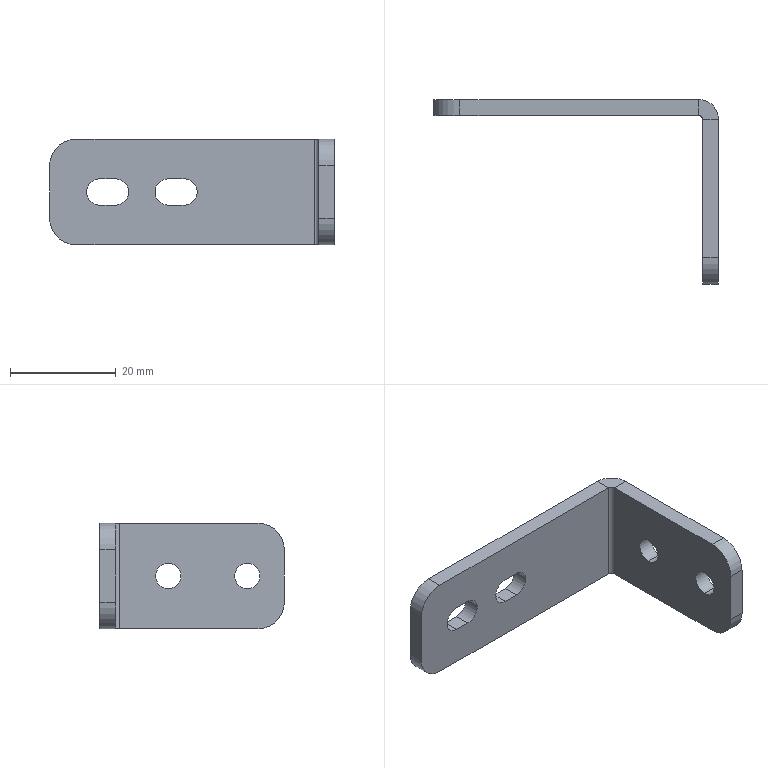Part | SolidWorks | features Fillet 1, FlatPattern 1, HoleWzd 1, ICE 1, SMBaseFlange 1, SheetMetal 1 | 1 solid | 30 faces | box 54 x 35 x 20 mm | volume 4722 mm3 | plane 16 | cylinder 14 | commonest cylinder face diameters 4.8 x4 5 x4 10 x4 1.473 x1 7.473 x1
STEP:
#1=CARTESIAN_POINT('',(54.,-13.,12.4));
#2=VERTEX_POINT('',#1);
#3=CARTESIAN_POINT('',(54.,-13.,7.6));
#4=VERTEX_POINT('',#3);
#5=CARTESIAN_POINT('',(54.,-13.,10.));
#6=DIRECTION('',(1.,0.,0.));
#7=DIRECTION('',(0.,1.,0.));
#8=AXIS2_PLACEMENT_3D('',#5,#6,#7);
#9=CIRCLE('',#8,2.4);
#10=EDGE_CURVE('',#2,#4,#9,.T.);
#11=ORIENTED_EDGE('',*,*,#10,.T.);
#12=CARTESIAN_POINT('',(51.,-13.,7.6));
#13=VERTEX_POINT('',#12);
#14=CARTESIAN_POINT('',(51.,-13.,7.6));
#15=DIRECTION('',(-1.,0.,0.));
#16=VECTOR('',#15,1000.);
#17=LINE('',#14,#16);
#18=EDGE_CURVE('',#4,#13,#17,.T.);
#19=ORIENTED_EDGE('',*,*,#18,.T.);
#20=CARTESIAN_POINT('',(51.,-13.,12.4));
#21=VERTEX_POINT('',#20);
#22=CARTESIAN_POINT('',(51.,-13.,10.));
#23=DIRECTION('',(-1.,0.,0.));
#24=DIRECTION('',(0.,0.,1.));
#25=AXIS2_PLACEMENT_3D('',#22,#23,#24);
#26=CIRCLE('',#25,2.4);
#27=EDGE_CURVE('',#13,#21,#26,.T.);
#28=ORIENTED_EDGE('',*,*,#27,.T.);
#29=CARTESIAN_POINT('',(51.,-13.,12.4));
#30=DIRECTION('',(-1.,0.,0.));
#31=VECTOR('',#30,1000.);
#32=LINE('',#29,#31);
#33=EDGE_CURVE('',#2,#21,#32,.T.);
#34=ORIENTED_EDGE('',*,*,#33,.F.);
#35=EDGE_LOOP('',(#11,#19,#28,#34));
#36=FACE_OUTER_BOUND('',#35,.T.);
#37=CARTESIAN_POINT('',(51.,-13.,10.));
#38=DIRECTION('',(-1.,0.,0.));
#39=DIRECTION('',(0.,0.,1.));
#40=AXIS2_PLACEMENT_3D('',#37,#38,#39);
#41=CYLINDRICAL_SURFACE('',#40,2.4);
#42=ADVANCED_FACE('',(#36),#41,.F.);
#43=CARTESIAN_POINT('',(54.,-28.,12.4));
#44=VERTEX_POINT('',#43);
#45=CARTESIAN_POINT('',(54.,-28.,7.6));
#46=VERTEX_POINT('',#45);
#47=CARTESIAN_POINT('',(54.,-28.,10.));
#48=DIRECTION('',(1.,0.,0.));
#49=DIRECTION('',(0.,1.,0.));
#50=AXIS2_PLACEMENT_3D('',#47,#48,#49);
#51=CIRCLE('',#50,2.4);
#52=EDGE_CURVE('',#44,#46,#51,.T.);
#53=ORIENTED_EDGE('',*,*,#52,.T.);
#54=CARTESIAN_POINT('',(51.,-28.,7.6));
#55=VERTEX_POINT('',#54);
#56=CARTESIAN_POINT('',(51.,-28.,7.6));
#57=DIRECTION('',(-1.,0.,0.));
#58=VECTOR('',#57,1000.);
#59=LINE('',#56,#58);
#60=EDGE_CURVE('',#46,#55,#59,.T.);
#61=ORIENTED_EDGE('',*,*,#60,.T.);
#62=CARTESIAN_POINT('',(51.,-28.,12.4));
#63=VERTEX_POINT('',#62);
#64=CARTESIAN_POINT('',(51.,-28.,10.));
#65=DIRECTION('',(-1.,0.,0.));
#66=DIRECTION('',(0.,0.,1.));
#67=AXIS2_PLACEMENT_3D('',#64,#65,#66);
#68=CIRCLE('',#67,2.4);
#69=EDGE_CURVE('',#55,#63,#68,.T.);
#70=ORIENTED_EDGE('',*,*,#69,.T.);
#71=CARTESIAN_POINT('',(51.,-28.,12.4));
#72=DIRECTION('',(-1.,0.,0.));
#73=VECTOR('',#72,1000.);
#74=LINE('',#71,#73);
#75=EDGE_CURVE('',#44,#63,#74,.T.);
#76=ORIENTED_EDGE('',*,*,#75,.F.);
#77=EDGE_LOOP('',(#53,#61,#70,#76));
#78=FACE_OUTER_BOUND('',#77,.T.);
#79=CARTESIAN_POINT('',(51.,-28.,10.));
#80=DIRECTION('',(-1.,0.,0.));
#81=DIRECTION('',(0.,0.,1.));
#82=AXIS2_PLACEMENT_3D('',#79,#80,#81);
#83=CYLINDRICAL_SURFACE('',#82,2.4);
#84=ADVANCED_FACE('',(#78),#83,.F.);
#85=CARTESIAN_POINT('',(54.,-3.737,20.));
#86=VERTEX_POINT('',#85);
#87=CARTESIAN_POINT('',(51.,-3.737,20.));
#88=VERTEX_POINT('',#87);
#89=CARTESIAN_POINT('',(54.,-3.737,20.));
#90=DIRECTION('',(-1.,0.,0.));
#91=VECTOR('',#90,1000.);
#92=LINE('',#89,#91);
#93=EDGE_CURVE('',#86,#88,#92,.T.);
#94=ORIENTED_EDGE('',*,*,#93,.F.);
#95=CARTESIAN_POINT('',(50.263,0.,20.));
#96=VERTEX_POINT('',#95);
#97=CARTESIAN_POINT('',(50.263,-3.737,20.));
#98=DIRECTION('',(0.,0.,-1.));
#99=DIRECTION('',(1.,0.,0.));
#100=AXIS2_PLACEMENT_3D('',#97,#98,#99);
#101=CIRCLE('',#100,3.737);
#102=EDGE_CURVE('',#96,#86,#101,.T.);
#103=ORIENTED_EDGE('',*,*,#102,.F.);
#104=CARTESIAN_POINT('',(50.263,-3.,20.));
#105=VERTEX_POINT('',#104);
#106=CARTESIAN_POINT('',(50.263,-3.,20.));
#107=DIRECTION('',(0.,1.,0.));
#108=VECTOR('',#107,1000.);
#109=LINE('',#106,#108);
#110=EDGE_CURVE('',#105,#96,#109,.T.);
#111=ORIENTED_EDGE('',*,*,#110,.F.);
#112=CARTESIAN_POINT('',(50.263,-3.737,20.));
#113=DIRECTION('',(0.,0.,-1.));
#114=DIRECTION('',(1.,0.,0.));
#115=AXIS2_PLACEMENT_3D('',#112,#113,#114);
#116=CIRCLE('',#115,0.7366);
#117=EDGE_CURVE('',#105,#88,#116,.T.);
#118=ORIENTED_EDGE('',*,*,#117,.T.);
#119=EDGE_LOOP('',(#94,#103,#111,#118));
#120=FACE_OUTER_BOUND('',#119,.T.);
#121=CARTESIAN_POINT('',(54.,-3.737,20.));
#122=DIRECTION('',(0.,0.,1.));
#123=DIRECTION('',(1.,0.,0.));
#124=AXIS2_PLACEMENT_3D('',#121,#122,#123);
#125=PLANE('',#124);
#126=ADVANCED_FACE('',(#120),#125,.T.);
#127=CARTESIAN_POINT('',(51.,-30.,20.));
#128=VERTEX_POINT('',#127);
#129=CARTESIAN_POINT('',(51.,0.,20.));
#130=DIRECTION('',(0.,-1.,0.));
#131=VECTOR('',#130,1000.);
#132=LINE('',#129,#131);
#133=EDGE_CURVE('',#88,#128,#132,.T.);
#134=ORIENTED_EDGE('',*,*,#133,.T.);
#135=CARTESIAN_POINT('',(54.,-30.,20.));
#136=VERTEX_POINT('',#135);
#137=CARTESIAN_POINT('',(50.263,-30.,20.));
#138=DIRECTION('',(1.,0.,0.));
#139=VECTOR('',#138,1000.);
#140=LINE('',#137,#139);
#141=EDGE_CURVE('',#128,#136,#140,.T.);
#142=ORIENTED_EDGE('',*,*,#141,.T.);
#143=CARTESIAN_POINT('',(54.,0.,20.));
#144=DIRECTION('',(0.,-1.,0.));
#145=VECTOR('',#144,1000.);
#146=LINE('',#143,#145);
#147=EDGE_CURVE('',#86,#136,#146,.T.);
#148=ORIENTED_EDGE('',*,*,#147,.F.);
#149=ORIENTED_EDGE('',*,*,#93,.T.);
#150=EDGE_LOOP('',(#134,#142,#148,#149));
#151=FACE_OUTER_BOUND('',#150,.T.);
#152=CARTESIAN_POINT('',(50.263,-3.,20.));
#153=DIRECTION('',(0.,0.,1.));
#154=DIRECTION('',(1.,0.,0.));
#155=AXIS2_PLACEMENT_3D('',#152,#153,#154);
#156=PLANE('',#155);
#157=ADVANCED_FACE('',(#151),#156,.T.);
#158=CARTESIAN_POINT('',(50.263,0.,0.));
#159=VERTEX_POINT('',#158);
#160=CARTESIAN_POINT('',(50.263,-3.,0.));
#161=VERTEX_POINT('',#160);
#162=CARTESIAN_POINT('',(50.263,0.,0.));
#163=DIRECTION('',(0.,-1.,0.));
#164=VECTOR('',#163,1000.);
#165=LINE('',#162,#164);
#166=EDGE_CURVE('',#159,#161,#165,.T.);
#167=ORIENTED_EDGE('',*,*,#166,.F.);
#168=CARTESIAN_POINT('',(54.,-3.737,0.));
#169=VERTEX_POINT('',#168);
#170=CARTESIAN_POINT('',(50.263,-3.737,0.));
#171=DIRECTION('',(0.,0.,-1.));
#172=DIRECTION('',(1.,0.,0.));
#173=AXIS2_PLACEMENT_3D('',#170,#171,#172);
#174=CIRCLE('',#173,3.737);
#175=EDGE_CURVE('',#159,#169,#174,.T.);
#176=ORIENTED_EDGE('',*,*,#175,.T.);
#177=CARTESIAN_POINT('',(51.,-3.737,0.));
#178=VERTEX_POINT('',#177);
#179=CARTESIAN_POINT('',(51.,-3.737,0.));
#180=DIRECTION('',(1.,0.,0.));
#181=VECTOR('',#180,1000.);
#182=LINE('',#179,#181);
#183=EDGE_CURVE('',#178,#169,#182,.T.);
#184=ORIENTED_EDGE('',*,*,#183,.F.);
#185=CARTESIAN_POINT('',(50.263,-3.737,0.));
#186=DIRECTION('',(0.,0.,-1.));
#187=DIRECTION('',(1.,0.,0.));
#188=AXIS2_PLACEMENT_3D('',#185,#186,#187);
#189=CIRCLE('',#188,0.7366);
#190=EDGE_CURVE('',#161,#178,#189,.T.);
#191=ORIENTED_EDGE('',*,*,#190,.F.);
#192=EDGE_LOOP('',(#167,#176,#184,#191));
#193=FACE_OUTER_BOUND('',#192,.T.);
#194=CARTESIAN_POINT('',(50.263,0.,0.));
#195=DIRECTION('',(0.,0.,-1.));
#196=DIRECTION('',(-1.,0.,0.));
#197=AXIS2_PLACEMENT_3D('',#194,#195,#196);
#198=PLANE('',#197);
#199=ADVANCED_FACE('',(#193),#198,.T.);
#200=CARTESIAN_POINT('',(5.,-3.,0.));
#201=VERTEX_POINT('',#200);
#202=CARTESIAN_POINT('',(0.,-3.,0.));
#203=DIRECTION('',(1.,0.,0.));
#204=VECTOR('',#203,1000.);
#205=LINE('',#202,#204);
#206=EDGE_CURVE('',#201,#161,#205,.T.);
#207=ORIENTED_EDGE('',*,*,#206,.F.);
#208=CARTESIAN_POINT('',(5.,0.,0.));
#209=VERTEX_POINT('',#208);
#210=CARTESIAN_POINT('',(5.,-3.737,0.));
#211=DIRECTION('',(0.,1.,0.));
#212=VECTOR('',#211,1000.);
#213=LINE('',#210,#212);
#214=EDGE_CURVE('',#201,#209,#213,.T.);
#215=ORIENTED_EDGE('',*,*,#214,.T.);
#216=CARTESIAN_POINT('',(0.,0.,0.));
#217=DIRECTION('',(1.,0.,0.));
#218=VECTOR('',#217,1000.);
#219=LINE('',#216,#218);
#220=EDGE_CURVE('',#209,#159,#219,.T.);
#221=ORIENTED_EDGE('',*,*,#220,.T.);
#222=ORIENTED_EDGE('',*,*,#166,.T.);
#223=EDGE_LOOP('',(#207,#215,#221,#222));
#224=FACE_OUTER_BOUND('',#223,.T.);
#225=CARTESIAN_POINT('',(51.,-3.737,0.));
#226=DIRECTION('',(0.,0.,-1.));
#227=DIRECTION('',(-1.,0.,0.));
#228=AXIS2_PLACEMENT_3D('',#225,#226,#227);
#229=PLANE('',#228);
#230=ADVANCED_FACE('',(#224),#229,.T.);
#231=CARTESIAN_POINT('',(51.,-13.,10.));
#232=DIRECTION('',(-1.,0.,0.));
#233=DIRECTION('',(0.,0.,1.));
#234=AXIS2_PLACEMENT_3D('',#231,#232,#233);
#235=CIRCLE('',#234,2.4);
#236=EDGE_CURVE('',#21,#13,#235,.T.);
#237=ORIENTED_EDGE('',*,*,#236,.F.);
#238=ORIENTED_EDGE('',*,*,#27,.F.);
#239=EDGE_LOOP('',(#237,#238));
#240=FACE_BOUND('',#239,.T.);
#241=CARTESIAN_POINT('',(51.,-28.,10.));
#242=DIRECTION('',(-1.,0.,0.));
#243=DIRECTION('',(0.,0.,1.));
#244=AXIS2_PLACEMENT_3D('',#241,#242,#243);
#245=CIRCLE('',#244,2.4);
#246=EDGE_CURVE('',#63,#55,#245,.T.);
#247=ORIENTED_EDGE('',*,*,#246,.F.);
#248=ORIENTED_EDGE('',*,*,#69,.F.);
#249=EDGE_LOOP('',(#247,#248));
#250=FACE_BOUND('',#249,.T.);
#251=CARTESIAN_POINT('',(51.,-35.,15.));
#252=VERTEX_POINT('',#251);
#253=CARTESIAN_POINT('',(51.,-35.,5.));
#254=VERTEX_POINT('',#253);
#255=CARTESIAN_POINT('',(51.,-35.,20.));
#256=DIRECTION('',(0.,0.,-1.));
#257=VECTOR('',#256,1000.);
#258=LINE('',#255,#257);
#259=EDGE_CURVE('',#252,#254,#258,.T.);
#260=ORIENTED_EDGE('',*,*,#259,.F.);
#261=CARTESIAN_POINT('',(51.,-30.,15.));
#262=DIRECTION('',(-1.,0.,0.));
#263=DIRECTION('',(0.,1.,0.));
#264=AXIS2_PLACEMENT_3D('',#261,#262,#263);
#265=CIRCLE('',#264,5.);
#266=EDGE_CURVE('',#252,#128,#265,.T.);
#267=ORIENTED_EDGE('',*,*,#266,.T.);
#268=ORIENTED_EDGE('',*,*,#133,.F.);
#269=CARTESIAN_POINT('',(51.,-3.737,20.));
#270=DIRECTION('',(0.,0.,-1.));
#271=VECTOR('',#270,1000.);
#272=LINE('',#269,#271);
#273=EDGE_CURVE('',#88,#178,#272,.T.);
#274=ORIENTED_EDGE('',*,*,#273,.T.);
#275=CARTESIAN_POINT('',(51.,-30.,0.));
#276=VERTEX_POINT('',#275);
#277=CARTESIAN_POINT('',(51.,0.,0.));
#278=DIRECTION('',(0.,-1.,0.));
#279=VECTOR('',#278,1000.);
#280=LINE('',#277,#279);
#281=EDGE_CURVE('',#178,#276,#280,.T.);
#282=ORIENTED_EDGE('',*,*,#281,.T.);
#283=CARTESIAN_POINT('',(51.,-30.,5.));
#284=DIRECTION('',(-1.,0.,0.));
#285=DIRECTION('',(0.,1.,0.));
#286=AXIS2_PLACEMENT_3D('',#283,#284,#285);
#287=CIRCLE('',#286,5.);
#288=EDGE_CURVE('',#276,#254,#287,.T.);
#289=ORIENTED_EDGE('',*,*,#288,.T.);
#290=EDGE_LOOP('',(#260,#267,#268,#274,#282,#289));
#291=FACE_OUTER_BOUND('',#290,.T.);
#292=CARTESIAN_POINT('',(51.,0.,20.));
#293=DIRECTION('',(1.,0.,0.));
#294=DIRECTION('',(0.,1.,0.));
#295=AXIS2_PLACEMENT_3D('',#292,#293,#294);
#296=PLANE('',#295);
#297=ADVANCED_FACE('',(#240,#250,#291),#296,.F.);
#298=CARTESIAN_POINT('',(54.,-35.,15.));
#299=VERTEX_POINT('',#298);
#300=CARTESIAN_POINT('',(54.,-35.,5.));
#301=VERTEX_POINT('',#300);
#302=CARTESIAN_POINT('',(54.,-35.,20.));
#303=DIRECTION('',(0.,0.,-1.));
#304=VECTOR('',#303,1000.);
#305=LINE('',#302,#304);
#306=EDGE_CURVE('',#299,#301,#305,.T.);
#307=ORIENTED_EDGE('',*,*,#306,.F.);
#308=CARTESIAN_POINT('',(54.,-35.,15.));
#309=DIRECTION('',(-1.,0.,0.));
#310=VECTOR('',#309,1000.);
#311=LINE('',#308,#310);
#312=EDGE_CURVE('',#299,#252,#311,.T.);
#313=ORIENTED_EDGE('',*,*,#312,.T.);
#314=ORIENTED_EDGE('',*,*,#259,.T.);
#315=CARTESIAN_POINT('',(54.,-35.,5.));
#316=DIRECTION('',(1.,0.,0.));
#317=VECTOR('',#316,1000.);
#318=LINE('',#315,#317);
#319=EDGE_CURVE('',#254,#301,#318,.T.);
#320=ORIENTED_EDGE('',*,*,#319,.T.);
#321=EDGE_LOOP('',(#307,#313,#314,#320));
#322=FACE_OUTER_BOUND('',#321,.T.);
#323=CARTESIAN_POINT('',(54.,-35.,20.));
#324=DIRECTION('',(0.,-1.,0.));
#325=DIRECTION('',(0.,0.,-1.));
#326=AXIS2_PLACEMENT_3D('',#323,#324,#325);
#327=PLANE('',#326);
#328=ADVANCED_FACE('',(#322),#327,.T.);
#329=ORIENTED_EDGE('',*,*,#10,.F.);
#330=CARTESIAN_POINT('',(54.,-13.,10.));
#331=DIRECTION('',(1.,0.,0.));
#332=DIRECTION('',(0.,1.,0.));
#333=AXIS2_PLACEMENT_3D('',#330,#331,#332);
#334=CIRCLE('',#333,2.4);
#335=EDGE_CURVE('',#4,#2,#334,.T.);
#336=ORIENTED_EDGE('',*,*,#335,.F.);
#337=EDGE_LOOP('',(#329,#336));
#338=FACE_BOUND('',#337,.T.);
#339=ORIENTED_EDGE('',*,*,#52,.F.);
#340=CARTESIAN_POINT('',(54.,-28.,10.));
#341=DIRECTION('',(1.,0.,0.));
#342=DIRECTION('',(0.,1.,0.));
#343=AXIS2_PLACEMENT_3D('',#340,#341,#342);
#344=CIRCLE('',#343,2.4);
#345=EDGE_CURVE('',#46,#44,#344,.T.);
#346=ORIENTED_EDGE('',*,*,#345,.F.);
#347=EDGE_LOOP('',(#339,#346));
#348=FACE_BOUND('',#347,.T.);
#349=ORIENTED_EDGE('',*,*,#147,.T.);
#350=CARTESIAN_POINT('',(54.,-30.,15.));
#351=DIRECTION('',(1.,0.,0.));
#352=DIRECTION('',(0.,1.,0.));
#353=AXIS2_PLACEMENT_3D('',#350,#351,#352);
#354=CIRCLE('',#353,5.);
#355=EDGE_CURVE('',#136,#299,#354,.T.);
#356=ORIENTED_EDGE('',*,*,#355,.T.);
#357=ORIENTED_EDGE('',*,*,#306,.T.);
#358=CARTESIAN_POINT('',(54.,-30.,0.));
#359=VERTEX_POINT('',#358);
#360=CARTESIAN_POINT('',(54.,-30.,5.));
#361=DIRECTION('',(1.,0.,0.));
#362=DIRECTION('',(0.,1.,0.));
#363=AXIS2_PLACEMENT_3D('',#360,#361,#362);
#364=CIRCLE('',#363,5.);
#365=EDGE_CURVE('',#301,#359,#364,.T.);
#366=ORIENTED_EDGE('',*,*,#365,.T.);
#367=CARTESIAN_POINT('',(54.,0.,0.));
#368=DIRECTION('',(0.,-1.,0.));
#369=VECTOR('',#368,1000.);
#370=LINE('',#367,#369);
#371=EDGE_CURVE('',#169,#359,#370,.T.);
#372=ORIENTED_EDGE('',*,*,#371,.F.);
#373=CARTESIAN_POINT('',(54.,-3.737,20.));
#374=DIRECTION('',(0.,0.,-1.));
#375=VECTOR('',#374,1000.);
#376=LINE('',#373,#375);
#377=EDGE_CURVE('',#86,#169,#376,.T.);
#378=ORIENTED_EDGE('',*,*,#377,.F.);
#379=EDGE_LOOP('',(#349,#356,#357,#366,#372,#378));
#380=FACE_OUTER_BOUND('',#379,.T.);
#381=CARTESIAN_POINT('',(54.,0.,20.));
#382=DIRECTION('',(1.,0.,0.));
#383=DIRECTION('',(0.,1.,0.));
#384=AXIS2_PLACEMENT_3D('',#381,#382,#383);
#385=PLANE('',#384);
#386=ADVANCED_FACE('',(#338,#348,#380),#385,.T.);
#387=ORIENTED_EDGE('',*,*,#175,.F.);
#388=CARTESIAN_POINT('',(50.263,0.,20.));
#389=DIRECTION('',(0.,0.,-1.));
#390=VECTOR('',#389,1000.);
#391=LINE('',#388,#390);
#392=EDGE_CURVE('',#96,#159,#391,.T.);
#393=ORIENTED_EDGE('',*,*,#392,.F.);
#394=ORIENTED_EDGE('',*,*,#102,.T.);
#395=ORIENTED_EDGE('',*,*,#377,.T.);
#396=EDGE_LOOP('',(#387,#393,#394,#395));
#397=FACE_OUTER_BOUND('',#396,.T.);
#398=CARTESIAN_POINT('',(50.263,-3.737,20.));
#399=DIRECTION('',(0.,0.,-1.));
#400=DIRECTION('',(-1.,0.,0.));
#401=AXIS2_PLACEMENT_3D('',#398,#399,#400);
#402=CYLINDRICAL_SURFACE('',#401,3.737);
#403=ADVANCED_FACE('',(#397),#402,.T.);
#404=CARTESIAN_POINT('',(9.5,0.,7.5));
#405=VERTEX_POINT('',#404);
#406=CARTESIAN_POINT('',(9.5,0.,12.5));
#407=VERTEX_POINT('',#406);
#408=CARTESIAN_POINT('',(9.5,0.,10.));
#409=DIRECTION('',(0.,1.,0.));
#410=DIRECTION('',(0.,0.,1.));
#411=AXIS2_PLACEMENT_3D('',#408,#409,#410);
#412=CIRCLE('',#411,2.5);
#413=EDGE_CURVE('',#405,#407,#412,.T.);
#414=ORIENTED_EDGE('',*,*,#413,.F.);
#415=CARTESIAN_POINT('',(12.5,0.,7.5));
#416=VERTEX_POINT('',#415);
#417=CARTESIAN_POINT('',(9.5,0.,7.5));
#418=DIRECTION('',(-1.,0.,0.));
#419=VECTOR('',#418,1000.);
#420=LINE('',#417,#419);
#421=EDGE_CURVE('',#416,#405,#420,.T.);
#422=ORIENTED_EDGE('',*,*,#421,.F.);
#423=CARTESIAN_POINT('',(12.5,0.,12.5));
#424=VERTEX_POINT('',#423);
#425=CARTESIAN_POINT('',(12.5,0.,10.));
#426=DIRECTION('',(0.,1.,0.));
#427=DIRECTION('',(0.,0.,1.));
#428=AXIS2_PLACEMENT_3D('',#425,#426,#427);
#429=CIRCLE('',#428,2.5);
#430=EDGE_CURVE('',#424,#416,#429,.T.);
#431=ORIENTED_EDGE('',*,*,#430,.F.);
#432=CARTESIAN_POINT('',(9.5,0.,12.5));
#433=DIRECTION('',(1.,0.,0.));
#434=VECTOR('',#433,1000.);
#435=LINE('',#432,#434);
#436=EDGE_CURVE('',#407,#424,#435,.T.);
#437=ORIENTED_EDGE('',*,*,#436,.F.);
#438=EDGE_LOOP('',(#414,#422,#431,#437));
#439=FACE_BOUND('',#438,.T.);
#440=CARTESIAN_POINT('',(25.5,0.,12.5));
#441=VERTEX_POINT('',#440);
#442=CARTESIAN_POINT('',(25.5,0.,7.5));
#443=VERTEX_POINT('',#442);
#444=CARTESIAN_POINT('',(25.5,0.,10.));
#445=DIRECTION('',(0.,1.,0.));
#446=DIRECTION('',(0.,0.,-1.));
#447=AXIS2_PLACEMENT_3D('',#444,#445,#446);
#448=CIRCLE('',#447,2.5);
#449=EDGE_CURVE('',#441,#443,#448,.T.);
#450=ORIENTED_EDGE('',*,*,#449,.F.);
#451=CARTESIAN_POINT('',(22.5,0.,12.5));
#452=VERTEX_POINT('',#451);
#453=CARTESIAN_POINT('',(25.5,0.,12.5));
#454=DIRECTION('',(1.,0.,0.));
#455=VECTOR('',#454,1000.);
#456=LINE('',#453,#455);
#457=EDGE_CURVE('',#452,#441,#456,.T.);
#458=ORIENTED_EDGE('',*,*,#457,.F.);
#459=CARTESIAN_POINT('',(22.5,0.,7.5));
#460=VERTEX_POINT('',#459);
#461=CARTESIAN_POINT('',(22.5,0.,10.));
#462=DIRECTION('',(0.,1.,0.));
#463=DIRECTION('',(0.,0.,-1.));
#464=AXIS2_PLACEMENT_3D('',#461,#462,#463);
#465=CIRCLE('',#464,2.5);
#466=EDGE_CURVE('',#460,#452,#465,.T.);
#467=ORIENTED_EDGE('',*,*,#466,.F.);
#468=CARTESIAN_POINT('',(25.5,0.,7.5));
#469=DIRECTION('',(-1.,0.,0.));
#470=VECTOR('',#469,1000.);
#471=LINE('',#468,#470);
#472=EDGE_CURVE('',#443,#460,#471,.T.);
#473=ORIENTED_EDGE('',*,*,#472,.F.);
#474=EDGE_LOOP('',(#450,#458,#467,#473));
#475=FACE_BOUND('',#474,.T.);
#476=CARTESIAN_POINT('',(0.,0.,15.));
#477=VERTEX_POINT('',#476);
#478=CARTESIAN_POINT('',(0.,0.,5.));
#479=VERTEX_POINT('',#478);
#480=CARTESIAN_POINT('',(0.,0.,20.));
#481=DIRECTION('',(0.,0.,-1.));
#482=VECTOR('',#481,1000.);
#483=LINE('',#480,#482);
#484=EDGE_CURVE('',#477,#479,#483,.T.);
#485=ORIENTED_EDGE('',*,*,#484,.F.);
#486=CARTESIAN_POINT('',(5.,0.,20.));
#487=VERTEX_POINT('',#486);
#488=CARTESIAN_POINT('',(5.,0.,15.));
#489=DIRECTION('',(0.,1.,0.));
#490=DIRECTION('',(0.,0.,1.));
#491=AXIS2_PLACEMENT_3D('',#488,#489,#490);
#492=CIRCLE('',#491,5.);
#493=EDGE_CURVE('',#477,#487,#492,.T.);
#494=ORIENTED_EDGE('',*,*,#493,.T.);
#495=CARTESIAN_POINT('',(0.,0.,20.));
#496=DIRECTION('',(1.,0.,0.));
#497=VECTOR('',#496,1000.);
#498=LINE('',#495,#497);
#499=EDGE_CURVE('',#487,#96,#498,.T.);
#500=ORIENTED_EDGE('',*,*,#499,.T.);
#501=ORIENTED_EDGE('',*,*,#392,.T.);
#502=ORIENTED_EDGE('',*,*,#220,.F.);
#503=CARTESIAN_POINT('',(5.,0.,5.));
#504=DIRECTION('',(0.,1.,0.));
#505=DIRECTION('',(0.,0.,1.));
#506=AXIS2_PLACEMENT_3D('',#503,#504,#505);
#507=CIRCLE('',#506,5.);
#508=EDGE_CURVE('',#209,#479,#507,.T.);
#509=ORIENTED_EDGE('',*,*,#508,.T.);
#510=EDGE_LOOP('',(#485,#494,#500,#501,#502,#509));
#511=FACE_OUTER_BOUND('',#510,.T.);
#512=CARTESIAN_POINT('',(0.,0.,20.));
#513=DIRECTION('',(0.,1.,0.));
#514=DIRECTION('',(0.,0.,1.));
#515=AXIS2_PLACEMENT_3D('',#512,#513,#514);
#516=PLANE('',#515);
#517=ADVANCED_FACE('',(#439,#475,#511),#516,.T.);
#518=CARTESIAN_POINT('',(0.,-3.,15.));
#519=VERTEX_POINT('',#518);
#520=CARTESIAN_POINT('',(0.,-3.,5.));
#521=VERTEX_POINT('',#520);
#522=CARTESIAN_POINT('',(0.,-3.,20.));
#523=DIRECTION('',(0.,0.,-1.));
#524=VECTOR('',#523,1000.);
#525=LINE('',#522,#524);
#526=EDGE_CURVE('',#519,#521,#525,.T.);
#527=ORIENTED_EDGE('',*,*,#526,.F.);
#528=CARTESIAN_POINT('',(0.,-3.,15.));
#529=DIRECTION('',(0.,1.,0.));
#530=VECTOR('',#529,1000.);
#531=LINE('',#528,#530);
#532=EDGE_CURVE('',#519,#477,#531,.T.);
#533=ORIENTED_EDGE('',*,*,#532,.T.);
#534=ORIENTED_EDGE('',*,*,#484,.T.);
#535=CARTESIAN_POINT('',(0.,-3.,5.));
#536=DIRECTION('',(0.,-1.,0.));
#537=VECTOR('',#536,1000.);
#538=LINE('',#535,#537);
#539=EDGE_CURVE('',#479,#521,#538,.T.);
#540=ORIENTED_EDGE('',*,*,#539,.T.);
#541=EDGE_LOOP('',(#527,#533,#534,#540));
#542=FACE_OUTER_BOUND('',#541,.T.);
#543=CARTESIAN_POINT('',(0.,-3.,20.));
#544=DIRECTION('',(-1.,0.,0.));
#545=DIRECTION('',(0.,0.,1.));
#546=AXIS2_PLACEMENT_3D('',#543,#544,#545);
#547=PLANE('',#546);
#548=ADVANCED_FACE('',(#542),#547,.T.);
#549=CARTESIAN_POINT('',(12.5,-3.,7.5));
#550=VERTEX_POINT('',#549);
#551=CARTESIAN_POINT('',(9.5,-3.,7.5));
#552=VERTEX_POINT('',#551);
#553=CARTESIAN_POINT('',(0.,-3.,7.5));
#554=DIRECTION('',(-1.,0.,0.));
#555=VECTOR('',#554,1000.);
#556=LINE('',#553,#555);
#557=EDGE_CURVE('',#550,#552,#556,.T.);
#558=ORIENTED_EDGE('',*,*,#557,.T.);
#559=CARTESIAN_POINT('',(9.5,-3.,12.5));
#560=VERTEX_POINT('',#559);
#561=CARTESIAN_POINT('',(9.5,-3.,10.));
#562=DIRECTION('',(0.,1.,0.));
#563=DIRECTION('',(0.,0.,1.));
#564=AXIS2_PLACEMENT_3D('',#561,#562,#563);
#565=CIRCLE('',#564,2.5);
#566=EDGE_CURVE('',#552,#560,#565,.T.);
#567=ORIENTED_EDGE('',*,*,#566,.T.);
#568=CARTESIAN_POINT('',(12.5,-3.,12.5));
#569=VERTEX_POINT('',#568);
#570=CARTESIAN_POINT('',(0.,-3.,12.5));
#571=DIRECTION('',(1.,0.,0.));
#572=VECTOR('',#571,1000.);
#573=LINE('',#570,#572);
#574=EDGE_CURVE('',#560,#569,#573,.T.);
#575=ORIENTED_EDGE('',*,*,#574,.T.);
#576=CARTESIAN_POINT('',(12.5,-3.,10.));
#577=DIRECTION('',(0.,1.,0.));
#578=DIRECTION('',(0.,0.,1.));
#579=AXIS2_PLACEMENT_3D('',#576,#577,#578);
#580=CIRCLE('',#579,2.5);
#581=EDGE_CURVE('',#569,#550,#580,.T.);
#582=ORIENTED_EDGE('',*,*,#581,.T.);
#583=EDGE_LOOP('',(#558,#567,#575,#582));
#584=FACE_BOUND('',#583,.T.);
#585=CARTESIAN_POINT('',(22.5,-3.,12.5));
#586=VERTEX_POINT('',#585);
#587=CARTESIAN_POINT('',(25.5,-3.,12.5));
#588=VERTEX_POINT('',#587);
#589=CARTESIAN_POINT('',(0.,-3.,12.5));
#590=DIRECTION('',(1.,0.,0.));
#591=VECTOR('',#590,1000.);
#592=LINE('',#589,#591);
#593=EDGE_CURVE('',#586,#588,#592,.T.);
#594=ORIENTED_EDGE('',*,*,#593,.T.);
#595=CARTESIAN_POINT('',(25.5,-3.,7.5));
#596=VERTEX_POINT('',#595);
#597=CARTESIAN_POINT('',(25.5,-3.,10.));
#598=DIRECTION('',(0.,1.,0.));
#599=DIRECTION('',(0.,0.,1.));
#600=AXIS2_PLACEMENT_3D('',#597,#598,#599);
#601=CIRCLE('',#600,2.5);
#602=EDGE_CURVE('',#588,#596,#601,.T.);
#603=ORIENTED_EDGE('',*,*,#602,.T.);
#604=CARTESIAN_POINT('',(22.5,-3.,7.5));
#605=VERTEX_POINT('',#604);
#606=CARTESIAN_POINT('',(0.,-3.,7.5));
#607=DIRECTION('',(-1.,0.,0.));
#608=VECTOR('',#607,1000.);
#609=LINE('',#606,#608);
#610=EDGE_CURVE('',#596,#605,#609,.T.);
#611=ORIENTED_EDGE('',*,*,#610,.T.);
#612=CARTESIAN_POINT('',(22.5,-3.,10.));
#613=DIRECTION('',(0.,1.,0.));
#614=DIRECTION('',(0.,0.,1.));
#615=AXIS2_PLACEMENT_3D('',#612,#613,#614);
#616=CIRCLE('',#615,2.5);
#617=EDGE_CURVE('',#605,#586,#616,.T.);
#618=ORIENTED_EDGE('',*,*,#617,.T.);
#619=EDGE_LOOP('',(#594,#603,#611,#618));
#620=FACE_BOUND('',#619,.T.);
#621=CARTESIAN_POINT('',(5.,-3.,20.));
#622=VERTEX_POINT('',#621);
#623=CARTESIAN_POINT('',(0.,-3.,20.));
#624=DIRECTION('',(1.,0.,0.));
#625=VECTOR('',#624,1000.);
#626=LINE('',#623,#625);
#627=EDGE_CURVE('',#622,#105,#626,.T.);
#628=ORIENTED_EDGE('',*,*,#627,.F.);
#629=CARTESIAN_POINT('',(5.,-3.,15.));
#630=DIRECTION('',(0.,-1.,0.));
#631=DIRECTION('',(0.,0.,1.));
#632=AXIS2_PLACEMENT_3D('',#629,#630,#631);
#633=CIRCLE('',#632,5.);
#634=EDGE_CURVE('',#622,#519,#633,.T.);
#635=ORIENTED_EDGE('',*,*,#634,.T.);
#636=ORIENTED_EDGE('',*,*,#526,.T.);
#637=CARTESIAN_POINT('',(5.,-3.,5.));
#638=DIRECTION('',(0.,-1.,0.));
#639=DIRECTION('',(0.,0.,1.));
#640=AXIS2_PLACEMENT_3D('',#637,#638,#639);
#641=CIRCLE('',#640,5.);
#642=EDGE_CURVE('',#521,#201,#641,.T.);
#643=ORIENTED_EDGE('',*,*,#642,.T.);
#644=ORIENTED_EDGE('',*,*,#206,.T.);
#645=CARTESIAN_POINT('',(50.263,-3.,20.));
#646=DIRECTION('',(0.,0.,-1.));
#647=VECTOR('',#646,1000.);
#648=LINE('',#645,#647);
#649=EDGE_CURVE('',#105,#161,#648,.T.);
#650=ORIENTED_EDGE('',*,*,#649,.F.);
#651=EDGE_LOOP('',(#628,#635,#636,#643,#644,#650));
#652=FACE_OUTER_BOUND('',#651,.T.);
#653=CARTESIAN_POINT('',(0.,-3.,20.));
#654=DIRECTION('',(0.,1.,0.));
#655=DIRECTION('',(0.,0.,1.));
#656=AXIS2_PLACEMENT_3D('',#653,#654,#655);
#657=PLANE('',#656);
#658=ADVANCED_FACE('',(#584,#620,#652),#657,.F.);
#659=ORIENTED_EDGE('',*,*,#190,.T.);
#660=ORIENTED_EDGE('',*,*,#273,.F.);
#661=ORIENTED_EDGE('',*,*,#117,.F.);
#662=ORIENTED_EDGE('',*,*,#649,.T.);
#663=EDGE_LOOP('',(#659,#660,#661,#662));
#664=FACE_OUTER_BOUND('',#663,.T.);
#665=CARTESIAN_POINT('',(50.263,-3.737,20.));
#666=DIRECTION('',(0.,0.,-1.));
#667=DIRECTION('',(-1.,0.,0.));
#668=AXIS2_PLACEMENT_3D('',#665,#666,#667);
#669=CYLINDRICAL_SURFACE('',#668,0.7366);
#670=ADVANCED_FACE('',(#664),#669,.F.);
#671=ORIENTED_EDGE('',*,*,#499,.F.);
#672=CARTESIAN_POINT('',(5.,-3.737,20.));
#673=DIRECTION('',(0.,-1.,0.));
#674=VECTOR('',#673,1000.);
#675=LINE('',#672,#674);
#676=EDGE_CURVE('',#487,#622,#675,.T.);
#677=ORIENTED_EDGE('',*,*,#676,.T.);
#678=ORIENTED_EDGE('',*,*,#627,.T.);
#679=ORIENTED_EDGE('',*,*,#110,.T.);
#680=EDGE_LOOP('',(#671,#677,#678,#679));
#681=FACE_OUTER_BOUND('',#680,.T.);
#682=CARTESIAN_POINT('',(50.263,-3.737,20.));
#683=DIRECTION('',(0.,0.,1.));
#684=DIRECTION('',(1.,0.,0.));
#685=AXIS2_PLACEMENT_3D('',#682,#683,#684);
#686=PLANE('',#685);
#687=ADVANCED_FACE('',(#681),#686,.T.);
#688=ORIENTED_EDGE('',*,*,#371,.T.);
#689=CARTESIAN_POINT('',(51.,-30.,0.));
#690=DIRECTION('',(-1.,0.,0.));
#691=VECTOR('',#690,1000.);
#692=LINE('',#689,#691);
#693=EDGE_CURVE('',#359,#276,#692,.T.);
#694=ORIENTED_EDGE('',*,*,#693,.T.);
#695=ORIENTED_EDGE('',*,*,#281,.F.);
#696=ORIENTED_EDGE('',*,*,#183,.T.);
#697=EDGE_LOOP('',(#688,#694,#695,#696));
#698=FACE_OUTER_BOUND('',#697,.T.);
#699=CARTESIAN_POINT('',(50.263,-3.737,0.));
#700=DIRECTION('',(0.,0.,1.));
#701=DIRECTION('',(1.,0.,0.));
#702=AXIS2_PLACEMENT_3D('',#699,#700,#701);
#703=PLANE('',#702);
#704=ADVANCED_FACE('',(#698),#703,.F.);
#705=CARTESIAN_POINT('',(25.5,-35.,12.5));
#706=DIRECTION('',(0.,1.,0.));
#707=VECTOR('',#706,1000.);
#708=LINE('',#705,#707);
#709=EDGE_CURVE('',#588,#441,#708,.T.);
#710=ORIENTED_EDGE('',*,*,#709,.T.);
#711=ORIENTED_EDGE('',*,*,#449,.T.);
#712=CARTESIAN_POINT('',(25.5,-35.,7.5));
#713=DIRECTION('',(0.,1.,0.));
#714=VECTOR('',#713,1000.);
#715=LINE('',#712,#714);
#716=EDGE_CURVE('',#596,#443,#715,.T.);
#717=ORIENTED_EDGE('',*,*,#716,.F.);
#718=ORIENTED_EDGE('',*,*,#602,.F.);
#719=EDGE_LOOP('',(#710,#711,#717,#718));
#720=FACE_OUTER_BOUND('',#719,.T.);
#721=CARTESIAN_POINT('',(25.5,-35.,10.));
#722=DIRECTION('',(0.,1.,0.));
#723=DIRECTION('',(0.,0.,1.));
#724=AXIS2_PLACEMENT_3D('',#721,#722,#723);
#725=CYLINDRICAL_SURFACE('',#724,2.5);
#726=ADVANCED_FACE('',(#720),#725,.F.);
#727=CARTESIAN_POINT('',(22.5,-35.,12.5));
#728=DIRECTION('',(0.,1.,0.));
#729=VECTOR('',#728,1000.);
#730=LINE('',#727,#729);
#731=EDGE_CURVE('',#586,#452,#730,.T.);
#732=ORIENTED_EDGE('',*,*,#731,.T.);
#733=ORIENTED_EDGE('',*,*,#457,.T.);
#734=ORIENTED_EDGE('',*,*,#709,.F.);
#735=ORIENTED_EDGE('',*,*,#593,.F.);
#736=EDGE_LOOP('',(#732,#733,#734,#735));
#737=FACE_OUTER_BOUND('',#736,.T.);
#738=CARTESIAN_POINT('',(25.5,-35.,12.5));
#739=DIRECTION('',(0.,0.,1.));
#740=DIRECTION('',(1.,0.,0.));
#741=AXIS2_PLACEMENT_3D('',#738,#739,#740);
#742=PLANE('',#741);
#743=ADVANCED_FACE('',(#737),#742,.F.);
#744=CARTESIAN_POINT('',(22.5,-35.,7.5));
#745=DIRECTION('',(0.,1.,0.));
#746=VECTOR('',#745,1000.);
#747=LINE('',#744,#746);
#748=EDGE_CURVE('',#605,#460,#747,.T.);
#749=ORIENTED_EDGE('',*,*,#748,.T.);
#750=ORIENTED_EDGE('',*,*,#466,.T.);
#751=ORIENTED_EDGE('',*,*,#731,.F.);
#752=ORIENTED_EDGE('',*,*,#617,.F.);
#753=EDGE_LOOP('',(#749,#750,#751,#752));
#754=FACE_OUTER_BOUND('',#753,.T.);
#755=CARTESIAN_POINT('',(22.5,-35.,10.));
#756=DIRECTION('',(0.,1.,0.));
#757=DIRECTION('',(0.,0.,1.));
#758=AXIS2_PLACEMENT_3D('',#755,#756,#757);
#759=CYLINDRICAL_SURFACE('',#758,2.5);
#760=ADVANCED_FACE('',(#754),#759,.F.);
#761=ORIENTED_EDGE('',*,*,#716,.T.);
#762=ORIENTED_EDGE('',*,*,#472,.T.);
#763=ORIENTED_EDGE('',*,*,#748,.F.);
#764=ORIENTED_EDGE('',*,*,#610,.F.);
#765=EDGE_LOOP('',(#761,#762,#763,#764));
#766=FACE_OUTER_BOUND('',#765,.T.);
#767=CARTESIAN_POINT('',(25.5,-35.,7.5));
#768=DIRECTION('',(0.,0.,-1.));
#769=DIRECTION('',(-1.,0.,0.));
#770=AXIS2_PLACEMENT_3D('',#767,#768,#769);
#771=PLANE('',#770);
#772=ADVANCED_FACE('',(#766),#771,.F.);
#773=CARTESIAN_POINT('',(9.5,-35.,7.5));
#774=DIRECTION('',(0.,1.,0.));
#775=VECTOR('',#774,1000.);
#776=LINE('',#773,#775);
#777=EDGE_CURVE('',#552,#405,#776,.T.);
#778=ORIENTED_EDGE('',*,*,#777,.T.);
#779=ORIENTED_EDGE('',*,*,#413,.T.);
#780=CARTESIAN_POINT('',(9.5,-35.,12.5));
#781=DIRECTION('',(0.,1.,0.));
#782=VECTOR('',#781,1000.);
#783=LINE('',#780,#782);
#784=EDGE_CURVE('',#560,#407,#783,.T.);
#785=ORIENTED_EDGE('',*,*,#784,.F.);
#786=ORIENTED_EDGE('',*,*,#566,.F.);
#787=EDGE_LOOP('',(#778,#779,#785,#786));
#788=FACE_OUTER_BOUND('',#787,.T.);
#789=CARTESIAN_POINT('',(9.5,-35.,10.));
#790=DIRECTION('',(0.,1.,0.));
#791=DIRECTION('',(0.,0.,1.));
#792=AXIS2_PLACEMENT_3D('',#789,#790,#791);
#793=CYLINDRICAL_SURFACE('',#792,2.5);
#794=ADVANCED_FACE('',(#788),#793,.F.);
#795=CARTESIAN_POINT('',(12.5,-35.,7.5));
#796=DIRECTION('',(0.,1.,0.));
#797=VECTOR('',#796,1000.);
#798=LINE('',#795,#797);
#799=EDGE_CURVE('',#550,#416,#798,.T.);
#800=ORIENTED_EDGE('',*,*,#799,.T.);
#801=ORIENTED_EDGE('',*,*,#421,.T.);
#802=ORIENTED_EDGE('',*,*,#777,.F.);
#803=ORIENTED_EDGE('',*,*,#557,.F.);
#804=EDGE_LOOP('',(#800,#801,#802,#803));
#805=FACE_OUTER_BOUND('',#804,.T.);
#806=CARTESIAN_POINT('',(9.5,-35.,7.5));
#807=DIRECTION('',(0.,0.,-1.));
#808=DIRECTION('',(-1.,0.,0.));
#809=AXIS2_PLACEMENT_3D('',#806,#807,#808);
#810=PLANE('',#809);
#811=ADVANCED_FACE('',(#805),#810,.F.);
#812=CARTESIAN_POINT('',(12.5,-35.,12.5));
#813=DIRECTION('',(0.,1.,0.));
#814=VECTOR('',#813,1000.);
#815=LINE('',#812,#814);
#816=EDGE_CURVE('',#569,#424,#815,.T.);
#817=ORIENTED_EDGE('',*,*,#816,.T.);
#818=ORIENTED_EDGE('',*,*,#430,.T.);
#819=ORIENTED_EDGE('',*,*,#799,.F.);
#820=ORIENTED_EDGE('',*,*,#581,.F.);
#821=EDGE_LOOP('',(#817,#818,#819,#820));
#822=FACE_OUTER_BOUND('',#821,.T.);
#823=CARTESIAN_POINT('',(12.5,-35.,10.));
#824=DIRECTION('',(0.,1.,0.));
#825=DIRECTION('',(0.,0.,1.));
#826=AXIS2_PLACEMENT_3D('',#823,#824,#825);
#827=CYLINDRICAL_SURFACE('',#826,2.5);
#828=ADVANCED_FACE('',(#822),#827,.F.);
#829=ORIENTED_EDGE('',*,*,#784,.T.);
#830=ORIENTED_EDGE('',*,*,#436,.T.);
#831=ORIENTED_EDGE('',*,*,#816,.F.);
#832=ORIENTED_EDGE('',*,*,#574,.F.);
#833=EDGE_LOOP('',(#829,#830,#831,#832));
#834=FACE_OUTER_BOUND('',#833,.T.);
#835=CARTESIAN_POINT('',(9.5,-35.,12.5));
#836=DIRECTION('',(0.,0.,1.));
#837=DIRECTION('',(1.,0.,0.));
#838=AXIS2_PLACEMENT_3D('',#835,#836,#837);
#839=PLANE('',#838);
#840=ADVANCED_FACE('',(#834),#839,.F.);
#841=ORIENTED_EDGE('',*,*,#60,.F.);
#842=ORIENTED_EDGE('',*,*,#345,.T.);
#843=ORIENTED_EDGE('',*,*,#75,.T.);
#844=ORIENTED_EDGE('',*,*,#246,.T.);
#845=EDGE_LOOP('',(#841,#842,#843,#844));
#846=FACE_OUTER_BOUND('',#845,.T.);
#847=CARTESIAN_POINT('',(51.,-28.,10.));
#848=DIRECTION('',(-1.,0.,0.));
#849=DIRECTION('',(0.,0.,1.));
#850=AXIS2_PLACEMENT_3D('',#847,#848,#849);
#851=CYLINDRICAL_SURFACE('',#850,2.4);
#852=ADVANCED_FACE('',(#846),#851,.F.);
#853=ORIENTED_EDGE('',*,*,#18,.F.);
#854=ORIENTED_EDGE('',*,*,#335,.T.);
#855=ORIENTED_EDGE('',*,*,#33,.T.);
#856=ORIENTED_EDGE('',*,*,#236,.T.);
#857=EDGE_LOOP('',(#853,#854,#855,#856));
#858=FACE_OUTER_BOUND('',#857,.T.);
#859=CARTESIAN_POINT('',(51.,-13.,10.));
#860=DIRECTION('',(-1.,0.,0.));
#861=DIRECTION('',(0.,0.,1.));
#862=AXIS2_PLACEMENT_3D('',#859,#860,#861);
#863=CYLINDRICAL_SURFACE('',#862,2.4);
#864=ADVANCED_FACE('',(#858),#863,.F.);
#865=ORIENTED_EDGE('',*,*,#355,.F.);
#866=ORIENTED_EDGE('',*,*,#141,.F.);
#867=ORIENTED_EDGE('',*,*,#266,.F.);
#868=ORIENTED_EDGE('',*,*,#312,.F.);
#869=EDGE_LOOP('',(#865,#866,#867,#868));
#870=FACE_OUTER_BOUND('',#869,.T.);
#871=CARTESIAN_POINT('',(54.,-30.,15.));
#872=DIRECTION('',(-1.,0.,0.));
#873=DIRECTION('',(0.,0.,1.));
#874=AXIS2_PLACEMENT_3D('',#871,#872,#873);
#875=CYLINDRICAL_SURFACE('',#874,5.);
#876=ADVANCED_FACE('',(#870),#875,.T.);
#877=ORIENTED_EDGE('',*,*,#365,.F.);
#878=ORIENTED_EDGE('',*,*,#319,.F.);
#879=ORIENTED_EDGE('',*,*,#288,.F.);
#880=ORIENTED_EDGE('',*,*,#693,.F.);
#881=EDGE_LOOP('',(#877,#878,#879,#880));
#882=FACE_OUTER_BOUND('',#881,.T.);
#883=CARTESIAN_POINT('',(50.263,-30.,5.));
#884=DIRECTION('',(1.,0.,0.));
#885=DIRECTION('',(0.,0.,-1.));
#886=AXIS2_PLACEMENT_3D('',#883,#884,#885);
#887=CYLINDRICAL_SURFACE('',#886,5.);
#888=ADVANCED_FACE('',(#882),#887,.T.);
#889=ORIENTED_EDGE('',*,*,#634,.F.);
#890=ORIENTED_EDGE('',*,*,#676,.F.);
#891=ORIENTED_EDGE('',*,*,#493,.F.);
#892=ORIENTED_EDGE('',*,*,#532,.F.);
#893=EDGE_LOOP('',(#889,#890,#891,#892));
#894=FACE_OUTER_BOUND('',#893,.T.);
#895=CARTESIAN_POINT('',(5.,-3.,15.));
#896=DIRECTION('',(0.,1.,0.));
#897=DIRECTION('',(0.,0.,1.));
#898=AXIS2_PLACEMENT_3D('',#895,#896,#897);
#899=CYLINDRICAL_SURFACE('',#898,5.);
#900=ADVANCED_FACE('',(#894),#899,.T.);
#901=ORIENTED_EDGE('',*,*,#642,.F.);
#902=ORIENTED_EDGE('',*,*,#539,.F.);
#903=ORIENTED_EDGE('',*,*,#508,.F.);
#904=ORIENTED_EDGE('',*,*,#214,.F.);
#905=EDGE_LOOP('',(#901,#902,#903,#904));
#906=FACE_OUTER_BOUND('',#905,.T.);
#907=CARTESIAN_POINT('',(5.,-3.737,5.));
#908=DIRECTION('',(0.,1.,0.));
#909=DIRECTION('',(0.,0.,1.));
#910=AXIS2_PLACEMENT_3D('',#907,#908,#909);
#911=CYLINDRICAL_SURFACE('',#910,5.);
#912=ADVANCED_FACE('',(#906),#911,.T.);
#913=CLOSED_SHELL('',(#42,#84,#126,#157,#199,#230,#297,#328,#386,#403,#517,#548,#658,#670,#687,#704,#726,#743,#760,#772,#794,#811,#828,#840,#852,#864,#876,#888,#900,#912));
#914=MANIFOLD_SOLID_BREP('',#913);
#915=CARTESIAN_POINT('',(0.,0.,0.));
#916=DIRECTION('',(0.,0.,1.));
#917=DIRECTION('',(1.,0.,0.));
#918=AXIS2_PLACEMENT_3D('',#915,#916,#917);
#919=(LENGTH_UNIT()NAMED_UNIT(*)SI_UNIT(.MILLI.,.METRE.));
#920=UNCERTAINTY_MEASURE_WITH_UNIT(LENGTH_MEASURE(0.00001),#919,'','');
#921=(NAMED_UNIT(*)PLANE_ANGLE_UNIT()SI_UNIT($,.RADIAN.));
#922=(NAMED_UNIT(*)SI_UNIT($,.STERADIAN.)SOLID_ANGLE_UNIT());
#923=(GEOMETRIC_REPRESENTATION_CONTEXT(3)GLOBAL_UNCERTAINTY_ASSIGNED_CONTEXT((#920))GLOBAL_UNIT_ASSIGNED_CONTEXT((#919,#921,#922))REPRESENTATION_CONTEXT('',''));
#924=ADVANCED_BREP_SHAPE_REPRESENTATION('',(#914,#918),#923);